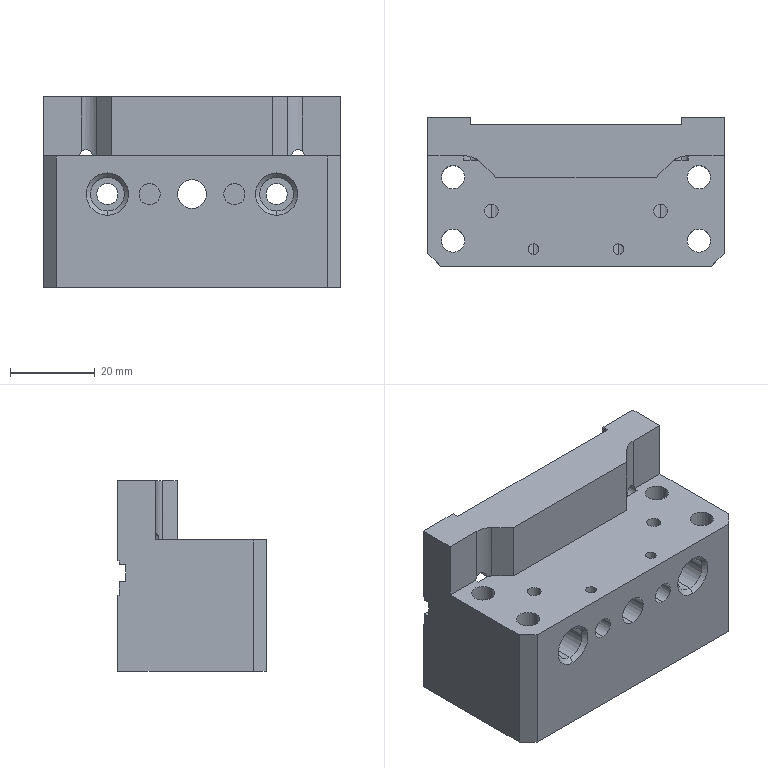Part | SolidWorks | features ICE 23, Chamfer 5, HoleWzd 5, 3DProfileFeature 3, Cut 2, Extrusion 1, Fillet 1, LPattern 1, MirrorPattern 1 | 1 solid | 140 faces | box 70 x 35 x 45 mm | volume 68698 mm3 | plane 64 | cylinder 58 | cone 18 | commonest cylinder face diameters 2.5 x12 3.3 x8 5 x8 5.5 x8 8 x8 3 x6